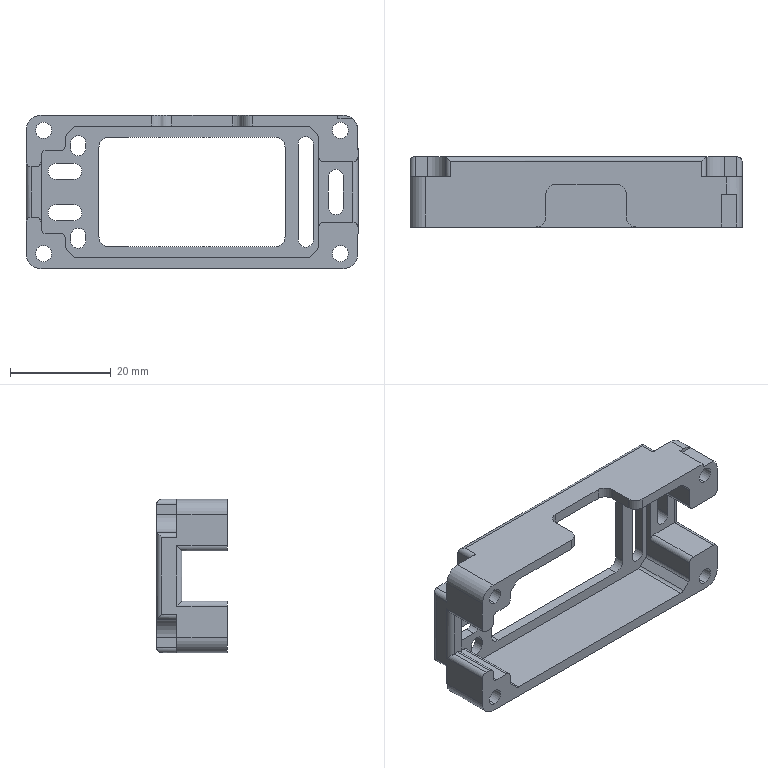Part | SolidWorks | features ICE 14, Fillet 6, Chamfer 1, Extrusion 1 | 1 solid | 135 faces | box 66 x 14 x 30.5 mm | volume 6792 mm3 | cylinder 74 | plane 61 | commonest cylinder face diameters 2 x34 3 x12 3.2 x12 4 x8 6 x4 7.2 x4